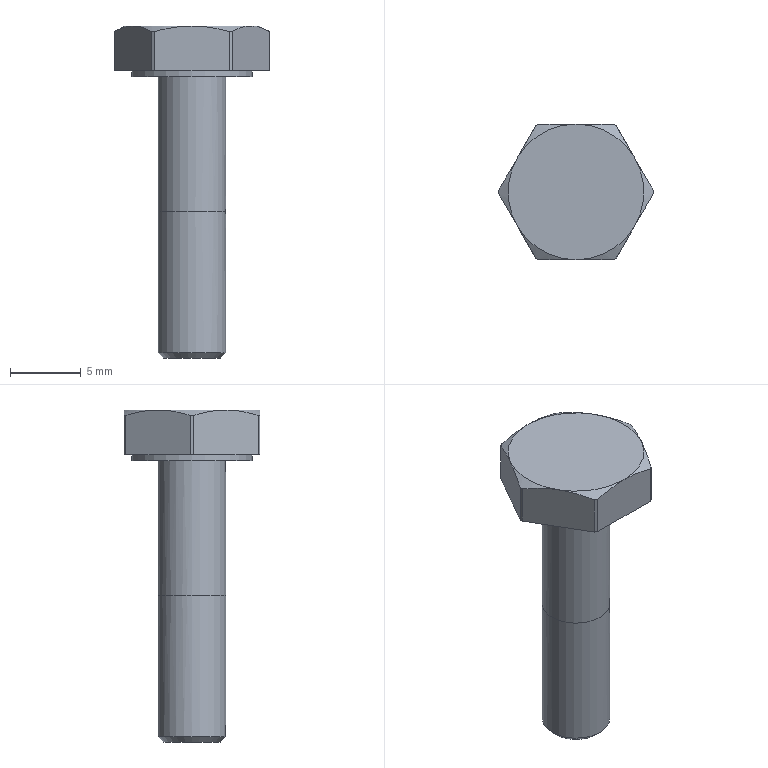Part | NX | features solid 2 | 1 solid | 26 faces | box 10.922 x 9.576 x 23.425 mm | volume 626.607 mm3 | plane 10 | cylinder 9 | cone 7 | commonest cylinder face diameters 10.922 x6 4.763 x2 8.509 x1
STEP:
#1=CARTESIAN_POINT('',(-2.381,0.,-3.581));
#2=VERTEX_POINT('',#1);
#3=CARTESIAN_POINT('',(0.,0.,-3.581));
#4=DIRECTION('',(0.,0.,-1.));
#5=DIRECTION('',(-1.,0.,0.));
#6=AXIS2_PLACEMENT_3D('',#3,#4,#5);
#7=CIRCLE('',#6,2.381);
#8=EDGE_CURVE('',#2,#2,#7,.T.);
#9=ORIENTED_EDGE('',*,*,#8,.T.);
#10=EDGE_LOOP('',(#9));
#11=FACE_BOUND('',#10,.T.);
#12=CARTESIAN_POINT('',(-2.381,0.,-13.106));
#13=VERTEX_POINT('',#12);
#14=CARTESIAN_POINT('',(-1.866,1.866,-13.106));
#15=CARTESIAN_POINT('',(-2.639,0.,-13.106));
#16=CARTESIAN_POINT('',(-1.866,-1.866,-13.106));
#17=CARTESIAN_POINT('',(0.,-2.639,-13.106));
#18=CARTESIAN_POINT('',(1.866,-1.866,-13.106));
#19=CARTESIAN_POINT('',(2.639,0.,-13.106));
#20=CARTESIAN_POINT('',(1.866,1.866,-13.106));
#21=CARTESIAN_POINT('',(0.,2.639,-13.106));
#22=CARTESIAN_POINT('',(-1.866,1.866,-13.106));
#23=CARTESIAN_POINT('',(-2.639,0.,-13.106));
#24=CARTESIAN_POINT('',(-1.866,-1.866,-13.106));
#25=B_SPLINE_CURVE_WITH_KNOTS('',3,(#14,#15,#16,#17,#18,#19,#20,#21,#22,#23,#24),.UNSPECIFIED.,.T.,.F.,(1,1,1,1,1,1,1,1,1,1,1,1,1,1,1),(-0.375,-0.25,-0.125,0.,0.125,0.25,0.375,0.5,0.625,0.75,0.875,1.,1.125,1.25,1.375),.UNSPECIFIED.);
#26=EDGE_CURVE('',#13,#13,#25,.T.);
#27=ORIENTED_EDGE('',*,*,#26,.T.);
#28=EDGE_LOOP('',(#27));
#29=FACE_BOUND('',#28,.T.);
#30=CARTESIAN_POINT('',(0.,0.,0.));
#31=DIRECTION('',(0.,0.,-1.));
#32=DIRECTION('',(-1.,0.,0.));
#33=AXIS2_PLACEMENT_3D('',#30,#31,#32);
#34=CYLINDRICAL_SURFACE('',#33,2.381);
#35=ADVANCED_FACE('',(#11,#29),#34,.T.);
#36=CARTESIAN_POINT('',(2.627,4.788,-3.175));
#37=VERTEX_POINT('',#36);
#38=CARTESIAN_POINT('',(2.833,4.669,-3.175));
#39=VERTEX_POINT('',#38);
#40=CARTESIAN_POINT('',(0.,0.,-3.175));
#41=DIRECTION('',(0.,0.,-1.));
#42=DIRECTION('',(-1.,0.,0.));
#43=AXIS2_PLACEMENT_3D('',#40,#41,#42);
#44=CIRCLE('',#43,5.461);
#45=EDGE_CURVE('',#37,#39,#44,.T.);
#46=ORIENTED_EDGE('',*,*,#45,.F.);
#47=CARTESIAN_POINT('',(2.627,4.788,-0.3886));
#48=VERTEX_POINT('',#47);
#49=CARTESIAN_POINT('',(2.627,4.788,0.));
#50=DIRECTION('',(0.,0.,-1.));
#51=VECTOR('',#50,1000.);
#52=LINE('',#49,#51);
#53=EDGE_CURVE('',#37,#48,#52,.F.);
#54=ORIENTED_EDGE('',*,*,#53,.T.);
#55=CARTESIAN_POINT('',(2.833,4.669,-0.3886));
#56=VERTEX_POINT('',#55);
#57=CARTESIAN_POINT('',(0.,0.,-0.3886));
#58=DIRECTION('',(0.,0.,-1.));
#59=DIRECTION('',(-1.,0.,0.));
#60=AXIS2_PLACEMENT_3D('',#57,#58,#59);
#61=CIRCLE('',#60,5.461);
#62=EDGE_CURVE('',#48,#56,#61,.T.);
#63=ORIENTED_EDGE('',*,*,#62,.T.);
#64=CARTESIAN_POINT('',(2.833,4.669,0.));
#65=DIRECTION('',(0.,0.,-1.));
#66=VECTOR('',#65,1000.);
#67=LINE('',#64,#66);
#68=EDGE_CURVE('',#56,#39,#67,.T.);
#69=ORIENTED_EDGE('',*,*,#68,.T.);
#70=EDGE_LOOP('',(#46,#54,#63,#69));
#71=FACE_BOUND('',#70,.T.);
#72=CARTESIAN_POINT('',(0.,0.,0.));
#73=DIRECTION('',(0.,0.,-1.));
#74=DIRECTION('',(-1.,0.,0.));
#75=AXIS2_PLACEMENT_3D('',#72,#73,#74);
#76=CYLINDRICAL_SURFACE('',#75,5.461);
#77=ADVANCED_FACE('',(#71),#76,.T.);
#78=CARTESIAN_POINT('',(-2.833,4.669,-0.3886));
#79=VERTEX_POINT('',#78);
#80=CARTESIAN_POINT('',(-2.627,4.788,-0.3886));
#81=VERTEX_POINT('',#80);
#82=CARTESIAN_POINT('',(0.,0.,-0.3886));
#83=DIRECTION('',(0.,0.,-1.));
#84=DIRECTION('',(-1.,0.,0.));
#85=AXIS2_PLACEMENT_3D('',#82,#83,#84);
#86=CIRCLE('',#85,5.461);
#87=EDGE_CURVE('',#79,#81,#86,.T.);
#88=ORIENTED_EDGE('',*,*,#87,.T.);
#89=CARTESIAN_POINT('',(-2.627,4.788,-3.175));
#90=VERTEX_POINT('',#89);
#91=CARTESIAN_POINT('',(-2.627,4.788,0.));
#92=DIRECTION('',(0.,0.,-1.));
#93=VECTOR('',#92,1000.);
#94=LINE('',#91,#93);
#95=EDGE_CURVE('',#81,#90,#94,.T.);
#96=ORIENTED_EDGE('',*,*,#95,.T.);
#97=CARTESIAN_POINT('',(-2.833,4.669,-3.175));
#98=VERTEX_POINT('',#97);
#99=CARTESIAN_POINT('',(0.,0.,-3.175));
#100=DIRECTION('',(0.,0.,-1.));
#101=DIRECTION('',(-1.,0.,0.));
#102=AXIS2_PLACEMENT_3D('',#99,#100,#101);
#103=CIRCLE('',#102,5.461);
#104=EDGE_CURVE('',#98,#90,#103,.T.);
#105=ORIENTED_EDGE('',*,*,#104,.F.);
#106=CARTESIAN_POINT('',(-2.833,4.669,0.));
#107=DIRECTION('',(0.,0.,-1.));
#108=VECTOR('',#107,1000.);
#109=LINE('',#106,#108);
#110=EDGE_CURVE('',#98,#79,#109,.F.);
#111=ORIENTED_EDGE('',*,*,#110,.T.);
#112=EDGE_LOOP('',(#88,#96,#105,#111));
#113=FACE_BOUND('',#112,.T.);
#114=CARTESIAN_POINT('',(0.,0.,0.));
#115=DIRECTION('',(0.,0.,-1.));
#116=DIRECTION('',(-1.,0.,0.));
#117=AXIS2_PLACEMENT_3D('',#114,#115,#116);
#118=CYLINDRICAL_SURFACE('',#117,5.461);
#119=ADVANCED_FACE('',(#113),#118,.T.);
#120=CARTESIAN_POINT('',(-5.46,-0.1193,-0.3886));
#121=VERTEX_POINT('',#120);
#122=CARTESIAN_POINT('',(-5.46,0.1193,-0.3886));
#123=VERTEX_POINT('',#122);
#124=CARTESIAN_POINT('',(0.,0.,-0.3886));
#125=DIRECTION('',(0.,0.,-1.));
#126=DIRECTION('',(-1.,0.,0.));
#127=AXIS2_PLACEMENT_3D('',#124,#125,#126);
#128=CIRCLE('',#127,5.461);
#129=EDGE_CURVE('',#121,#123,#128,.T.);
#130=ORIENTED_EDGE('',*,*,#129,.T.);
#131=CARTESIAN_POINT('',(-5.46,0.1193,-3.175));
#132=VERTEX_POINT('',#131);
#133=CARTESIAN_POINT('',(-5.46,0.1193,0.));
#134=DIRECTION('',(0.,0.,-1.));
#135=VECTOR('',#134,1000.);
#136=LINE('',#133,#135);
#137=EDGE_CURVE('',#123,#132,#136,.T.);
#138=ORIENTED_EDGE('',*,*,#137,.T.);
#139=CARTESIAN_POINT('',(-5.46,-0.1193,-3.175));
#140=VERTEX_POINT('',#139);
#141=CARTESIAN_POINT('',(0.,0.,-3.175));
#142=DIRECTION('',(0.,0.,-1.));
#143=DIRECTION('',(-1.,0.,0.));
#144=AXIS2_PLACEMENT_3D('',#141,#142,#143);
#145=CIRCLE('',#144,5.461);
#146=EDGE_CURVE('',#140,#132,#145,.T.);
#147=ORIENTED_EDGE('',*,*,#146,.F.);
#148=CARTESIAN_POINT('',(-5.46,-0.1193,0.));
#149=DIRECTION('',(0.,0.,-1.));
#150=VECTOR('',#149,1000.);
#151=LINE('',#148,#150);
#152=EDGE_CURVE('',#140,#121,#151,.F.);
#153=ORIENTED_EDGE('',*,*,#152,.T.);
#154=EDGE_LOOP('',(#130,#138,#147,#153));
#155=FACE_BOUND('',#154,.T.);
#156=CARTESIAN_POINT('',(0.,0.,0.));
#157=DIRECTION('',(0.,0.,-1.));
#158=DIRECTION('',(-1.,0.,0.));
#159=AXIS2_PLACEMENT_3D('',#156,#157,#158);
#160=CYLINDRICAL_SURFACE('',#159,5.461);
#161=ADVANCED_FACE('',(#155),#160,.T.);
#162=CARTESIAN_POINT('',(-2.627,-4.788,-0.3886));
#163=VERTEX_POINT('',#162);
#164=CARTESIAN_POINT('',(-2.833,-4.669,-0.3886));
#165=VERTEX_POINT('',#164);
#166=CARTESIAN_POINT('',(0.,0.,-0.3886));
#167=DIRECTION('',(0.,0.,-1.));
#168=DIRECTION('',(-1.,0.,0.));
#169=AXIS2_PLACEMENT_3D('',#166,#167,#168);
#170=CIRCLE('',#169,5.461);
#171=EDGE_CURVE('',#163,#165,#170,.T.);
#172=ORIENTED_EDGE('',*,*,#171,.T.);
#173=CARTESIAN_POINT('',(-2.833,-4.669,-3.175));
#174=VERTEX_POINT('',#173);
#175=CARTESIAN_POINT('',(-2.833,-4.669,0.));
#176=DIRECTION('',(0.,0.,-1.));
#177=VECTOR('',#176,1000.);
#178=LINE('',#175,#177);
#179=EDGE_CURVE('',#165,#174,#178,.T.);
#180=ORIENTED_EDGE('',*,*,#179,.T.);
#181=CARTESIAN_POINT('',(-2.627,-4.788,-3.175));
#182=VERTEX_POINT('',#181);
#183=CARTESIAN_POINT('',(0.,0.,-3.175));
#184=DIRECTION('',(0.,0.,-1.));
#185=DIRECTION('',(-1.,0.,0.));
#186=AXIS2_PLACEMENT_3D('',#183,#184,#185);
#187=CIRCLE('',#186,5.461);
#188=EDGE_CURVE('',#182,#174,#187,.T.);
#189=ORIENTED_EDGE('',*,*,#188,.F.);
#190=CARTESIAN_POINT('',(-2.627,-4.788,0.));
#191=DIRECTION('',(0.,0.,-1.));
#192=VECTOR('',#191,1000.);
#193=LINE('',#190,#192);
#194=EDGE_CURVE('',#182,#163,#193,.F.);
#195=ORIENTED_EDGE('',*,*,#194,.T.);
#196=EDGE_LOOP('',(#172,#180,#189,#195));
#197=FACE_BOUND('',#196,.T.);
#198=CARTESIAN_POINT('',(0.,0.,0.));
#199=DIRECTION('',(0.,0.,-1.));
#200=DIRECTION('',(-1.,0.,0.));
#201=AXIS2_PLACEMENT_3D('',#198,#199,#200);
#202=CYLINDRICAL_SURFACE('',#201,5.461);
#203=ADVANCED_FACE('',(#197),#202,.T.);
#204=CARTESIAN_POINT('',(2.833,-4.669,-0.3886));
#205=VERTEX_POINT('',#204);
#206=CARTESIAN_POINT('',(2.627,-4.788,-0.3886));
#207=VERTEX_POINT('',#206);
#208=CARTESIAN_POINT('',(0.,0.,-0.3886));
#209=DIRECTION('',(0.,0.,-1.));
#210=DIRECTION('',(-1.,0.,0.));
#211=AXIS2_PLACEMENT_3D('',#208,#209,#210);
#212=CIRCLE('',#211,5.461);
#213=EDGE_CURVE('',#205,#207,#212,.T.);
#214=ORIENTED_EDGE('',*,*,#213,.T.);
#215=CARTESIAN_POINT('',(2.627,-4.788,-3.175));
#216=VERTEX_POINT('',#215);
#217=CARTESIAN_POINT('',(2.627,-4.788,0.));
#218=DIRECTION('',(0.,0.,-1.));
#219=VECTOR('',#218,1000.);
#220=LINE('',#217,#219);
#221=EDGE_CURVE('',#207,#216,#220,.T.);
#222=ORIENTED_EDGE('',*,*,#221,.T.);
#223=CARTESIAN_POINT('',(2.833,-4.669,-3.175));
#224=VERTEX_POINT('',#223);
#225=CARTESIAN_POINT('',(0.,0.,-3.175));
#226=DIRECTION('',(0.,0.,-1.));
#227=DIRECTION('',(-1.,0.,0.));
#228=AXIS2_PLACEMENT_3D('',#225,#226,#227);
#229=CIRCLE('',#228,5.461);
#230=EDGE_CURVE('',#224,#216,#229,.T.);
#231=ORIENTED_EDGE('',*,*,#230,.F.);
#232=CARTESIAN_POINT('',(2.833,-4.669,0.));
#233=DIRECTION('',(0.,0.,-1.));
#234=VECTOR('',#233,1000.);
#235=LINE('',#232,#234);
#236=EDGE_CURVE('',#224,#205,#235,.F.);
#237=ORIENTED_EDGE('',*,*,#236,.T.);
#238=EDGE_LOOP('',(#214,#222,#231,#237));
#239=FACE_BOUND('',#238,.T.);
#240=CARTESIAN_POINT('',(0.,0.,0.));
#241=DIRECTION('',(0.,0.,-1.));
#242=DIRECTION('',(-1.,0.,0.));
#243=AXIS2_PLACEMENT_3D('',#240,#241,#242);
#244=CYLINDRICAL_SURFACE('',#243,5.461);
#245=ADVANCED_FACE('',(#239),#244,.T.);
#246=ORIENTED_EDGE('',*,*,#62,.F.);
#247=CARTESIAN_POINT('',(0.,4.788,0.));
#248=VERTEX_POINT('',#247);
#249=CARTESIAN_POINT('',(0.,4.788,0.));
#250=CARTESIAN_POINT('',(0.8868,4.788,0.));
#251=CARTESIAN_POINT('',(1.776,4.788,-0.1525));
#252=CARTESIAN_POINT('',(2.627,4.788,-0.3886));
#253=B_SPLINE_CURVE_WITH_KNOTS('',3,(#249,#250,#251,#252),.UNSPECIFIED.,.F.,.F.,(4,4),(0.007722,0.01038),.UNSPECIFIED.);
#254=EDGE_CURVE('',#48,#248,#253,.F.);
#255=ORIENTED_EDGE('',*,*,#254,.T.);
#256=CARTESIAN_POINT('',(4.146,2.394,0.));
#257=VERTEX_POINT('',#256);
#258=CARTESIAN_POINT('',(0.,0.,0.));
#259=DIRECTION('',(0.,0.,-1.));
#260=DIRECTION('',(-1.,0.,0.));
#261=AXIS2_PLACEMENT_3D('',#258,#259,#260);
#262=CIRCLE('',#261,4.788);
#263=EDGE_CURVE('',#248,#257,#262,.T.);
#264=ORIENTED_EDGE('',*,*,#263,.T.);
#265=CARTESIAN_POINT('',(4.146,2.394,0.));
#266=CARTESIAN_POINT('',(3.703,3.163,0.));
#267=CARTESIAN_POINT('',(3.262,3.925,-0.1503));
#268=CARTESIAN_POINT('',(2.833,4.669,-0.3886));
#269=B_SPLINE_CURVE_WITH_KNOTS('',3,(#265,#266,#267,#268),.UNSPECIFIED.,.F.,.F.,(4,4),(0.002655,0.005296),.UNSPECIFIED.);
#270=EDGE_CURVE('',#257,#56,#269,.T.);
#271=ORIENTED_EDGE('',*,*,#270,.T.);
#272=EDGE_LOOP('',(#246,#255,#264,#271));
#273=FACE_BOUND('',#272,.T.);
#274=CARTESIAN_POINT('',(0.,0.,-0.3886));
#275=DIRECTION('',(0.,0.,-1.));
#276=DIRECTION('',(-1.,0.,0.));
#277=AXIS2_PLACEMENT_3D('',#274,#275,#276);
#278=CONICAL_SURFACE('',#277,5.461,1.047);
#279=ADVANCED_FACE('',(#273),#278,.T.);
#280=CARTESIAN_POINT('',(-4.146,2.394,0.));
#281=VERTEX_POINT('',#280);
#282=CARTESIAN_POINT('',(0.,0.,0.));
#283=DIRECTION('',(0.,0.,-1.));
#284=DIRECTION('',(-1.,0.,0.));
#285=AXIS2_PLACEMENT_3D('',#282,#283,#284);
#286=CIRCLE('',#285,4.788);
#287=EDGE_CURVE('',#281,#248,#286,.T.);
#288=ORIENTED_EDGE('',*,*,#287,.T.);
#289=CARTESIAN_POINT('',(-2.627,4.788,-0.3886));
#290=CARTESIAN_POINT('',(-1.77,4.788,-0.1508));
#291=CARTESIAN_POINT('',(-0.8866,4.788,0.));
#292=CARTESIAN_POINT('',(0.,4.788,0.));
#293=B_SPLINE_CURVE_WITH_KNOTS('',3,(#289,#290,#291,#292),.UNSPECIFIED.,.F.,.F.,(4,4),(0.005068,0.007722),.UNSPECIFIED.);
#294=EDGE_CURVE('',#248,#81,#293,.F.);
#295=ORIENTED_EDGE('',*,*,#294,.T.);
#296=ORIENTED_EDGE('',*,*,#87,.F.);
#297=CARTESIAN_POINT('',(-2.833,4.669,-0.3886));
#298=CARTESIAN_POINT('',(-3.264,3.923,-0.1495));
#299=CARTESIAN_POINT('',(-3.7,3.167,0.));
#300=CARTESIAN_POINT('',(-4.146,2.394,0.));
#301=B_SPLINE_CURVE_WITH_KNOTS('',3,(#297,#298,#299,#300),.UNSPECIFIED.,.F.,.F.,(4,4),(0.00000074,0.002655),.UNSPECIFIED.);
#302=EDGE_CURVE('',#79,#281,#301,.T.);
#303=ORIENTED_EDGE('',*,*,#302,.T.);
#304=EDGE_LOOP('',(#288,#295,#296,#303));
#305=FACE_BOUND('',#304,.T.);
#306=CARTESIAN_POINT('',(0.,0.,-0.3886));
#307=DIRECTION('',(0.,0.,-1.));
#308=DIRECTION('',(-1.,0.,0.));
#309=AXIS2_PLACEMENT_3D('',#306,#307,#308);
#310=CONICAL_SURFACE('',#309,5.461,1.047);
#311=ADVANCED_FACE('',(#305),#310,.T.);
#312=CARTESIAN_POINT('',(-4.146,-2.394,0.));
#313=VERTEX_POINT('',#312);
#314=CARTESIAN_POINT('',(0.,0.,0.));
#315=DIRECTION('',(0.,0.,-1.));
#316=DIRECTION('',(-1.,0.,0.));
#317=AXIS2_PLACEMENT_3D('',#314,#315,#316);
#318=CIRCLE('',#317,4.788);
#319=EDGE_CURVE('',#313,#281,#318,.T.);
#320=ORIENTED_EDGE('',*,*,#319,.T.);
#321=CARTESIAN_POINT('',(-4.146,2.394,0.));
#322=CARTESIAN_POINT('',(-4.59,1.625,0.));
#323=CARTESIAN_POINT('',(-5.031,0.8625,-0.1503));
#324=CARTESIAN_POINT('',(-5.46,0.1193,-0.3886));
#325=B_SPLINE_CURVE_WITH_KNOTS('',3,(#321,#322,#323,#324),.UNSPECIFIED.,.F.,.F.,(4,4),(0.002655,0.005296),.UNSPECIFIED.);
#326=EDGE_CURVE('',#281,#123,#325,.T.);
#327=ORIENTED_EDGE('',*,*,#326,.T.);
#328=ORIENTED_EDGE('',*,*,#129,.F.);
#329=CARTESIAN_POINT('',(-5.46,-0.1193,-0.3886));
#330=CARTESIAN_POINT('',(-5.029,-0.8651,-0.1495));
#331=CARTESIAN_POINT('',(-4.593,-1.621,0.));
#332=CARTESIAN_POINT('',(-4.146,-2.394,0.));
#333=B_SPLINE_CURVE_WITH_KNOTS('',3,(#329,#330,#331,#332),.UNSPECIFIED.,.F.,.F.,(4,4),(0.00000074,0.002655),.UNSPECIFIED.);
#334=EDGE_CURVE('',#121,#313,#333,.T.);
#335=ORIENTED_EDGE('',*,*,#334,.T.);
#336=EDGE_LOOP('',(#320,#327,#328,#335));
#337=FACE_BOUND('',#336,.T.);
#338=CARTESIAN_POINT('',(0.,0.,-0.3886));
#339=DIRECTION('',(0.,0.,-1.));
#340=DIRECTION('',(-1.,0.,0.));
#341=AXIS2_PLACEMENT_3D('',#338,#339,#340);
#342=CONICAL_SURFACE('',#341,5.461,1.047);
#343=ADVANCED_FACE('',(#337),#342,.T.);
#344=CARTESIAN_POINT('',(0.,-4.788,0.));
#345=VERTEX_POINT('',#344);
#346=CARTESIAN_POINT('',(0.,0.,0.));
#347=DIRECTION('',(0.,0.,-1.));
#348=DIRECTION('',(-1.,0.,0.));
#349=AXIS2_PLACEMENT_3D('',#346,#347,#348);
#350=CIRCLE('',#349,4.788);
#351=EDGE_CURVE('',#345,#313,#350,.T.);
#352=ORIENTED_EDGE('',*,*,#351,.T.);
#353=CARTESIAN_POINT('',(-4.146,-2.394,0.));
#354=CARTESIAN_POINT('',(-3.703,-3.163,0.));
#355=CARTESIAN_POINT('',(-3.262,-3.925,-0.1503));
#356=CARTESIAN_POINT('',(-2.833,-4.669,-0.3886));
#357=B_SPLINE_CURVE_WITH_KNOTS('',3,(#353,#354,#355,#356),.UNSPECIFIED.,.F.,.F.,(4,4),(0.002655,0.005296),.UNSPECIFIED.);
#358=EDGE_CURVE('',#313,#165,#357,.T.);
#359=ORIENTED_EDGE('',*,*,#358,.T.);
#360=ORIENTED_EDGE('',*,*,#171,.F.);
#361=CARTESIAN_POINT('',(-2.627,-4.788,-0.3886));
#362=CARTESIAN_POINT('',(-1.77,-4.788,-0.1508));
#363=CARTESIAN_POINT('',(-0.8866,-4.788,0.));
#364=CARTESIAN_POINT('',(0.,-4.788,0.));
#365=B_SPLINE_CURVE_WITH_KNOTS('',3,(#361,#362,#363,#364),.UNSPECIFIED.,.F.,.F.,(4,4),(0.005068,0.007722),.UNSPECIFIED.);
#366=EDGE_CURVE('',#163,#345,#365,.T.);
#367=ORIENTED_EDGE('',*,*,#366,.T.);
#368=EDGE_LOOP('',(#352,#359,#360,#367));
#369=FACE_BOUND('',#368,.T.);
#370=CARTESIAN_POINT('',(0.,0.,-0.3886));
#371=DIRECTION('',(0.,0.,-1.));
#372=DIRECTION('',(-1.,0.,0.));
#373=AXIS2_PLACEMENT_3D('',#370,#371,#372);
#374=CONICAL_SURFACE('',#373,5.461,1.047);
#375=ADVANCED_FACE('',(#369),#374,.T.);
#376=CARTESIAN_POINT('',(4.146,-2.394,0.));
#377=VERTEX_POINT('',#376);
#378=CARTESIAN_POINT('',(0.,0.,0.));
#379=DIRECTION('',(0.,0.,-1.));
#380=DIRECTION('',(-1.,0.,0.));
#381=AXIS2_PLACEMENT_3D('',#378,#379,#380);
#382=CIRCLE('',#381,4.788);
#383=EDGE_CURVE('',#377,#345,#382,.T.);
#384=ORIENTED_EDGE('',*,*,#383,.T.);
#385=CARTESIAN_POINT('',(0.,-4.788,0.));
#386=CARTESIAN_POINT('',(0.8868,-4.788,0.));
#387=CARTESIAN_POINT('',(1.776,-4.788,-0.1525));
#388=CARTESIAN_POINT('',(2.627,-4.788,-0.3886));
#389=B_SPLINE_CURVE_WITH_KNOTS('',3,(#385,#386,#387,#388),.UNSPECIFIED.,.F.,.F.,(4,4),(0.007722,0.01038),.UNSPECIFIED.);
#390=EDGE_CURVE('',#345,#207,#389,.T.);
#391=ORIENTED_EDGE('',*,*,#390,.T.);
#392=ORIENTED_EDGE('',*,*,#213,.F.);
#393=CARTESIAN_POINT('',(2.833,-4.669,-0.3886));
#394=CARTESIAN_POINT('',(3.264,-3.923,-0.1495));
#395=CARTESIAN_POINT('',(3.7,-3.167,0.));
#396=CARTESIAN_POINT('',(4.146,-2.394,0.));
#397=B_SPLINE_CURVE_WITH_KNOTS('',3,(#393,#394,#395,#396),.UNSPECIFIED.,.F.,.F.,(4,4),(0.00000074,0.002655),.UNSPECIFIED.);
#398=EDGE_CURVE('',#205,#377,#397,.T.);
#399=ORIENTED_EDGE('',*,*,#398,.T.);
#400=EDGE_LOOP('',(#384,#391,#392,#399));
#401=FACE_BOUND('',#400,.T.);
#402=CARTESIAN_POINT('',(0.,0.,-0.3886));
#403=DIRECTION('',(0.,0.,-1.));
#404=DIRECTION('',(-1.,0.,0.));
#405=AXIS2_PLACEMENT_3D('',#402,#403,#404);
#406=CONICAL_SURFACE('',#405,5.461,1.047);
#407=ADVANCED_FACE('',(#401),#406,.T.);
#408=ORIENTED_EDGE('',*,*,#104,.T.);
#409=CARTESIAN_POINT('',(4.255,4.788,-3.175));
#410=DIRECTION('',(1.,0.,0.));
#411=VECTOR('',#410,1000.);
#412=LINE('',#409,#411);
#413=EDGE_CURVE('',#90,#37,#412,.T.);
#414=ORIENTED_EDGE('',*,*,#413,.T.);
#415=ORIENTED_EDGE('',*,*,#45,.T.);
#416=CARTESIAN_POINT('',(5.46,0.1193,-3.175));
#417=VERTEX_POINT('',#416);
#418=CARTESIAN_POINT('',(5.21,0.5517,-3.175));
#419=DIRECTION('',(0.5,-0.866,0.));
#420=VECTOR('',#419,1000.);
#421=LINE('',#418,#420);
#422=EDGE_CURVE('',#39,#417,#421,.T.);
#423=ORIENTED_EDGE('',*,*,#422,.T.);
#424=CARTESIAN_POINT('',(5.46,-0.1193,-3.175));
#425=VERTEX_POINT('',#424);
#426=CARTESIAN_POINT('',(0.,0.,-3.175));
#427=DIRECTION('',(0.,0.,-1.));
#428=DIRECTION('',(-1.,0.,0.));
#429=AXIS2_PLACEMENT_3D('',#426,#427,#428);
#430=CIRCLE('',#429,5.461);
#431=EDGE_CURVE('',#417,#425,#430,.T.);
#432=ORIENTED_EDGE('',*,*,#431,.T.);
#433=CARTESIAN_POINT('',(5.21,-0.5517,-3.175));
#434=DIRECTION('',(-0.5,-0.866,0.));
#435=VECTOR('',#434,1000.);
#436=LINE('',#433,#435);
#437=EDGE_CURVE('',#425,#224,#436,.T.);
#438=ORIENTED_EDGE('',*,*,#437,.T.);
#439=ORIENTED_EDGE('',*,*,#230,.T.);
#440=CARTESIAN_POINT('',(4.255,-4.788,-3.175));
#441=DIRECTION('',(-1.,0.,0.));
#442=VECTOR('',#441,1000.);
#443=LINE('',#440,#442);
#444=EDGE_CURVE('',#216,#182,#443,.T.);
#445=ORIENTED_EDGE('',*,*,#444,.T.);
#446=ORIENTED_EDGE('',*,*,#188,.T.);
#447=CARTESIAN_POINT('',(-3.083,-4.236,-3.175));
#448=DIRECTION('',(-0.5,0.866,0.));
#449=VECTOR('',#448,1000.);
#450=LINE('',#447,#449);
#451=EDGE_CURVE('',#174,#140,#450,.T.);
#452=ORIENTED_EDGE('',*,*,#451,.T.);
#453=ORIENTED_EDGE('',*,*,#146,.T.);
#454=CARTESIAN_POINT('',(-3.083,4.236,-3.175));
#455=DIRECTION('',(0.5,0.866,0.));
#456=VECTOR('',#455,1000.);
#457=LINE('',#454,#456);
#458=EDGE_CURVE('',#132,#98,#457,.T.);
#459=ORIENTED_EDGE('',*,*,#458,.T.);
#460=EDGE_LOOP('',(#408,#414,#415,#423,#432,#438,#439,#445,#446,#452,#453,#459));
#461=FACE_BOUND('',#460,.T.);
#462=CARTESIAN_POINT('',(-4.255,0.,-3.175));
#463=VERTEX_POINT('',#462);
#464=CARTESIAN_POINT('',(0.,0.,-3.175));
#465=DIRECTION('',(0.,0.,-1.));
#466=DIRECTION('',(-1.,0.,0.));
#467=AXIS2_PLACEMENT_3D('',#464,#465,#466);
#468=CIRCLE('',#467,4.255);
#469=EDGE_CURVE('',#463,#463,#468,.T.);
#470=ORIENTED_EDGE('',*,*,#469,.F.);
#471=EDGE_LOOP('',(#470));
#472=FACE_BOUND('',#471,.T.);
#473=CARTESIAN_POINT('',(4.255,0.,-3.175));
#474=DIRECTION('',(0.,0.,-1.));
#475=DIRECTION('',(-1.,0.,0.));
#476=AXIS2_PLACEMENT_3D('',#473,#474,#475);
#477=PLANE('',#476);
#478=ADVANCED_FACE('',(#461,#472),#477,.T.);
#479=CARTESIAN_POINT('',(5.46,0.1193,-0.3886));
#480=VERTEX_POINT('',#479);
#481=CARTESIAN_POINT('',(5.46,-0.1193,-0.3886));
#482=VERTEX_POINT('',#481);
#483=CARTESIAN_POINT('',(0.,0.,-0.3886));
#484=DIRECTION('',(0.,0.,-1.));
#485=DIRECTION('',(-1.,0.,0.));
#486=AXIS2_PLACEMENT_3D('',#483,#484,#485);
#487=CIRCLE('',#486,5.461);
#488=EDGE_CURVE('',#480,#482,#487,.T.);
#489=ORIENTED_EDGE('',*,*,#488,.T.);
#490=CARTESIAN_POINT('',(5.46,-0.1193,0.));
#491=DIRECTION('',(0.,0.,-1.));
#492=VECTOR('',#491,1000.);
#493=LINE('',#490,#492);
#494=EDGE_CURVE('',#482,#425,#493,.T.);
#495=ORIENTED_EDGE('',*,*,#494,.T.);
#496=ORIENTED_EDGE('',*,*,#431,.F.);
#497=CARTESIAN_POINT('',(5.46,0.1193,0.));
#498=DIRECTION('',(0.,0.,-1.));
#499=VECTOR('',#498,1000.);
#500=LINE('',#497,#499);
#501=EDGE_CURVE('',#417,#480,#500,.F.);
#502=ORIENTED_EDGE('',*,*,#501,.T.);
#503=EDGE_LOOP('',(#489,#495,#496,#502));
#504=FACE_BOUND('',#503,.T.);
#505=CARTESIAN_POINT('',(0.,0.,0.));
#506=DIRECTION('',(0.,0.,-1.));
#507=DIRECTION('',(-1.,0.,0.));
#508=AXIS2_PLACEMENT_3D('',#505,#506,#507);
#509=CYLINDRICAL_SURFACE('',#508,5.461);
#510=ADVANCED_FACE('',(#504),#509,.T.);
#511=CARTESIAN_POINT('',(0.,0.,0.));
#512=DIRECTION('',(0.,0.,-1.));
#513=DIRECTION('',(-1.,0.,0.));
#514=AXIS2_PLACEMENT_3D('',#511,#512,#513);
#515=CIRCLE('',#514,4.788);
#516=EDGE_CURVE('',#257,#377,#515,.T.);
#517=ORIENTED_EDGE('',*,*,#516,.T.);
#518=CARTESIAN_POINT('',(4.146,-2.394,0.));
#519=CARTESIAN_POINT('',(4.59,-1.625,0.));
#520=CARTESIAN_POINT('',(5.031,-0.8625,-0.1503));
#521=CARTESIAN_POINT('',(5.46,-0.1193,-0.3886));
#522=B_SPLINE_CURVE_WITH_KNOTS('',3,(#518,#519,#520,#521),.UNSPECIFIED.,.F.,.F.,(4,4),(0.002655,0.005296),.UNSPECIFIED.);
#523=EDGE_CURVE('',#377,#482,#522,.T.);
#524=ORIENTED_EDGE('',*,*,#523,.T.);
#525=ORIENTED_EDGE('',*,*,#488,.F.);
#526=CARTESIAN_POINT('',(5.46,0.1193,-0.3886));
#527=CARTESIAN_POINT('',(5.029,0.8651,-0.1495));
#528=CARTESIAN_POINT('',(4.593,1.621,0.));
#529=CARTESIAN_POINT('',(4.146,2.394,0.));
#530=B_SPLINE_CURVE_WITH_KNOTS('',3,(#526,#527,#528,#529),.UNSPECIFIED.,.F.,.F.,(4,4),(0.00000074,0.002655),.UNSPECIFIED.);
#531=EDGE_CURVE('',#480,#257,#530,.T.);
#532=ORIENTED_EDGE('',*,*,#531,.T.);
#533=EDGE_LOOP('',(#517,#524,#525,#532));
#534=FACE_BOUND('',#533,.T.);
#535=CARTESIAN_POINT('',(0.,0.,-0.3886));
#536=DIRECTION('',(0.,0.,-1.));
#537=DIRECTION('',(-1.,0.,0.));
#538=AXIS2_PLACEMENT_3D('',#535,#536,#537);
#539=CONICAL_SURFACE('',#538,5.461,1.047);
#540=ADVANCED_FACE('',(#534),#539,.T.);
#541=ORIENTED_EDGE('',*,*,#287,.F.);
#542=ORIENTED_EDGE('',*,*,#319,.F.);
#543=ORIENTED_EDGE('',*,*,#351,.F.);
#544=ORIENTED_EDGE('',*,*,#383,.F.);
#545=ORIENTED_EDGE('',*,*,#516,.F.);
#546=ORIENTED_EDGE('',*,*,#263,.F.);
#547=EDGE_LOOP('',(#541,#542,#543,#544,#545,#546));
#548=FACE_BOUND('',#547,.T.);
#549=CARTESIAN_POINT('',(4.788,0.,0.));
#550=DIRECTION('',(0.,0.,1.));
#551=DIRECTION('',(1.,0.,0.));
#552=AXIS2_PLACEMENT_3D('',#549,#550,#551);
#553=PLANE('',#552);
#554=ADVANCED_FACE('',(#548),#553,.T.);
#555=CARTESIAN_POINT('',(-2.,0.,-23.425));
#556=VERTEX_POINT('',#555);
#557=CARTESIAN_POINT('',(0.,0.,-23.425));
#558=DIRECTION('',(0.,0.,-1.));
#559=DIRECTION('',(-1.,0.,0.));
#560=AXIS2_PLACEMENT_3D('',#557,#558,#559);
#561=CIRCLE('',#560,2.);
#562=EDGE_CURVE('',#556,#556,#561,.T.);
#563=ORIENTED_EDGE('',*,*,#562,.T.);
#564=EDGE_LOOP('',(#563));
#565=FACE_BOUND('',#564,.T.);
#566=CARTESIAN_POINT('',(0.,0.,-23.425));
#567=DIRECTION('',(0.,0.,-1.));
#568=DIRECTION('',(-1.,0.,0.));
#569=AXIS2_PLACEMENT_3D('',#566,#567,#568);
#570=PLANE('',#569);
#571=ADVANCED_FACE('',(#565),#570,.T.);
#572=CARTESIAN_POINT('',(-2.381,0.,-23.044));
#573=VERTEX_POINT('',#572);
#574=CARTESIAN_POINT('',(0.,0.,-23.044));
#575=DIRECTION('',(0.,0.,-1.));
#576=DIRECTION('',(-1.,0.,0.));
#577=AXIS2_PLACEMENT_3D('',#574,#575,#576);
#578=CIRCLE('',#577,2.381);
#579=EDGE_CURVE('',#573,#573,#578,.T.);
#580=ORIENTED_EDGE('',*,*,#579,.T.);
#581=EDGE_LOOP('',(#580));
#582=FACE_BOUND('',#581,.T.);
#583=ORIENTED_EDGE('',*,*,#562,.F.);
#584=EDGE_LOOP('',(#583));
#585=FACE_BOUND('',#584,.T.);
#586=CARTESIAN_POINT('',(0.,0.,-23.425));
#587=DIRECTION('',(0.,0.,1.));
#588=DIRECTION('',(1.,0.,0.));
#589=AXIS2_PLACEMENT_3D('',#586,#587,#588);
#590=CONICAL_SURFACE('',#589,2.,0.7854);
#591=ADVANCED_FACE('',(#582,#585),#590,.T.);
#592=ORIENTED_EDGE('',*,*,#26,.F.);
#593=EDGE_LOOP('',(#592));
#594=FACE_BOUND('',#593,.T.);
#595=ORIENTED_EDGE('',*,*,#579,.F.);
#596=EDGE_LOOP('',(#595));
#597=FACE_BOUND('',#596,.T.);
#598=CARTESIAN_POINT('',(0.,0.,0.));
#599=DIRECTION('',(0.,0.,-1.));
#600=DIRECTION('',(-1.,0.,0.));
#601=AXIS2_PLACEMENT_3D('',#598,#599,#600);
#602=CYLINDRICAL_SURFACE('',#601,2.381);
#603=ADVANCED_FACE('',(#594,#597),#602,.T.);
#604=CARTESIAN_POINT('',(-4.255,0.,-3.581));
#605=VERTEX_POINT('',#604);
#606=CARTESIAN_POINT('',(0.,0.,-3.581));
#607=DIRECTION('',(0.,0.,-1.));
#608=DIRECTION('',(-1.,0.,0.));
#609=AXIS2_PLACEMENT_3D('',#606,#607,#608);
#610=CIRCLE('',#609,4.255);
#611=EDGE_CURVE('',#605,#605,#610,.T.);
#612=ORIENTED_EDGE('',*,*,#611,.T.);
#613=EDGE_LOOP('',(#612));
#614=FACE_BOUND('',#613,.T.);
#615=ORIENTED_EDGE('',*,*,#8,.F.);
#616=EDGE_LOOP('',(#615));
#617=FACE_BOUND('',#616,.T.);
#618=CARTESIAN_POINT('',(2.381,0.,-3.581));
#619=DIRECTION('',(0.,0.,-1.));
#620=DIRECTION('',(-1.,0.,0.));
#621=AXIS2_PLACEMENT_3D('',#618,#619,#620);
#622=PLANE('',#621);
#623=ADVANCED_FACE('',(#614,#617),#622,.T.);
#624=ORIENTED_EDGE('',*,*,#469,.T.);
#625=EDGE_LOOP('',(#624));
#626=FACE_BOUND('',#625,.T.);
#627=ORIENTED_EDGE('',*,*,#611,.F.);
#628=EDGE_LOOP('',(#627));
#629=FACE_BOUND('',#628,.T.);
#630=CARTESIAN_POINT('',(0.,0.,0.));
#631=DIRECTION('',(0.,0.,-1.));
#632=DIRECTION('',(-1.,0.,0.));
#633=AXIS2_PLACEMENT_3D('',#630,#631,#632);
#634=CYLINDRICAL_SURFACE('',#633,4.255);
#635=ADVANCED_FACE('',(#626,#629),#634,.T.);
#636=ORIENTED_EDGE('',*,*,#422,.F.);
#637=ORIENTED_EDGE('',*,*,#68,.F.);
#638=ORIENTED_EDGE('',*,*,#270,.F.);
#639=ORIENTED_EDGE('',*,*,#531,.F.);
#640=ORIENTED_EDGE('',*,*,#501,.F.);
#641=EDGE_LOOP('',(#636,#637,#638,#639,#640));
#642=FACE_BOUND('',#641,.T.);
#643=CARTESIAN_POINT('',(5.529,0.,-25.768));
#644=DIRECTION('',(0.866,0.5,0.));
#645=DIRECTION('',(-0.5,0.866,0.));
#646=AXIS2_PLACEMENT_3D('',#643,#644,#645);
#647=PLANE('',#646);
#648=ADVANCED_FACE('',(#642),#647,.T.);
#649=ORIENTED_EDGE('',*,*,#437,.F.);
#650=ORIENTED_EDGE('',*,*,#494,.F.);
#651=ORIENTED_EDGE('',*,*,#523,.F.);
#652=ORIENTED_EDGE('',*,*,#398,.F.);
#653=ORIENTED_EDGE('',*,*,#236,.F.);
#654=EDGE_LOOP('',(#649,#650,#651,#652,#653));
#655=FACE_BOUND('',#654,.T.);
#656=CARTESIAN_POINT('',(2.764,-4.788,-25.768));
#657=DIRECTION('',(0.866,-0.5,0.));
#658=DIRECTION('',(0.5,0.866,0.));
#659=AXIS2_PLACEMENT_3D('',#656,#657,#658);
#660=PLANE('',#659);
#661=ADVANCED_FACE('',(#655),#660,.T.);
#662=ORIENTED_EDGE('',*,*,#444,.F.);
#663=ORIENTED_EDGE('',*,*,#221,.F.);
#664=ORIENTED_EDGE('',*,*,#390,.F.);
#665=ORIENTED_EDGE('',*,*,#366,.F.);
#666=ORIENTED_EDGE('',*,*,#194,.F.);
#667=EDGE_LOOP('',(#662,#663,#664,#665,#666));
#668=FACE_BOUND('',#667,.T.);
#669=CARTESIAN_POINT('',(-2.764,-4.788,-25.768));
#670=DIRECTION('',(0.,-1.,0.));
#671=DIRECTION('',(0.,0.,-1.));
#672=AXIS2_PLACEMENT_3D('',#669,#670,#671);
#673=PLANE('',#672);
#674=ADVANCED_FACE('',(#668),#673,.T.);
#675=ORIENTED_EDGE('',*,*,#451,.F.);
#676=ORIENTED_EDGE('',*,*,#179,.F.);
#677=ORIENTED_EDGE('',*,*,#358,.F.);
#678=ORIENTED_EDGE('',*,*,#334,.F.);
#679=ORIENTED_EDGE('',*,*,#152,.F.);
#680=EDGE_LOOP('',(#675,#676,#677,#678,#679));
#681=FACE_BOUND('',#680,.T.);
#682=CARTESIAN_POINT('',(-5.529,0.,-25.768));
#683=DIRECTION('',(-0.866,-0.5,0.));
#684=DIRECTION('',(0.5,-0.866,0.));
#685=AXIS2_PLACEMENT_3D('',#682,#683,#684);
#686=PLANE('',#685);
#687=ADVANCED_FACE('',(#681),#686,.T.);
#688=ORIENTED_EDGE('',*,*,#458,.F.);
#689=ORIENTED_EDGE('',*,*,#137,.F.);
#690=ORIENTED_EDGE('',*,*,#326,.F.);
#691=ORIENTED_EDGE('',*,*,#302,.F.);
#692=ORIENTED_EDGE('',*,*,#110,.F.);
#693=EDGE_LOOP('',(#688,#689,#690,#691,#692));
#694=FACE_BOUND('',#693,.T.);
#695=CARTESIAN_POINT('',(-2.764,4.788,-25.768));
#696=DIRECTION('',(-0.866,0.5,0.));
#697=DIRECTION('',(-0.5,-0.866,0.));
#698=AXIS2_PLACEMENT_3D('',#695,#696,#697);
#699=PLANE('',#698);
#700=ADVANCED_FACE('',(#694),#699,.T.);
#701=ORIENTED_EDGE('',*,*,#413,.F.);
#702=ORIENTED_EDGE('',*,*,#95,.F.);
#703=ORIENTED_EDGE('',*,*,#294,.F.);
#704=ORIENTED_EDGE('',*,*,#254,.F.);
#705=ORIENTED_EDGE('',*,*,#53,.F.);
#706=EDGE_LOOP('',(#701,#702,#703,#704,#705));
#707=FACE_BOUND('',#706,.T.);
#708=CARTESIAN_POINT('',(2.764,4.788,-25.768));
#709=DIRECTION('',(0.,1.,0.));
#710=DIRECTION('',(0.,0.,1.));
#711=AXIS2_PLACEMENT_3D('',#708,#709,#710);
#712=PLANE('',#711);
#713=ADVANCED_FACE('',(#707),#712,.T.);
#714=CLOSED_SHELL('',(#35,#77,#119,#161,#203,#245,#279,#311,#343,#375,#407,#478,#510,#540,#554,#571,#591,#603,#623,#635,#648,#661,#674,#687,#700,#713));
#715=MANIFOLD_SOLID_BREP('',#714);
#716=(LENGTH_UNIT()NAMED_UNIT(*)SI_UNIT(.MILLI.,.METRE.));
#717=UNCERTAINTY_MEASURE_WITH_UNIT(LENGTH_MEASURE(0.0508),#716,'','');
#718=(NAMED_UNIT(*)PLANE_ANGLE_UNIT()SI_UNIT($,.RADIAN.));
#719=(NAMED_UNIT(*)SI_UNIT($,.STERADIAN.)SOLID_ANGLE_UNIT());
#720=(GEOMETRIC_REPRESENTATION_CONTEXT(3)GLOBAL_UNCERTAINTY_ASSIGNED_CONTEXT((#717))GLOBAL_UNIT_ASSIGNED_CONTEXT((#716,#718,#719))REPRESENTATION_CONTEXT('',''));
#721=ADVANCED_BREP_SHAPE_REPRESENTATION('',(#715),#720);